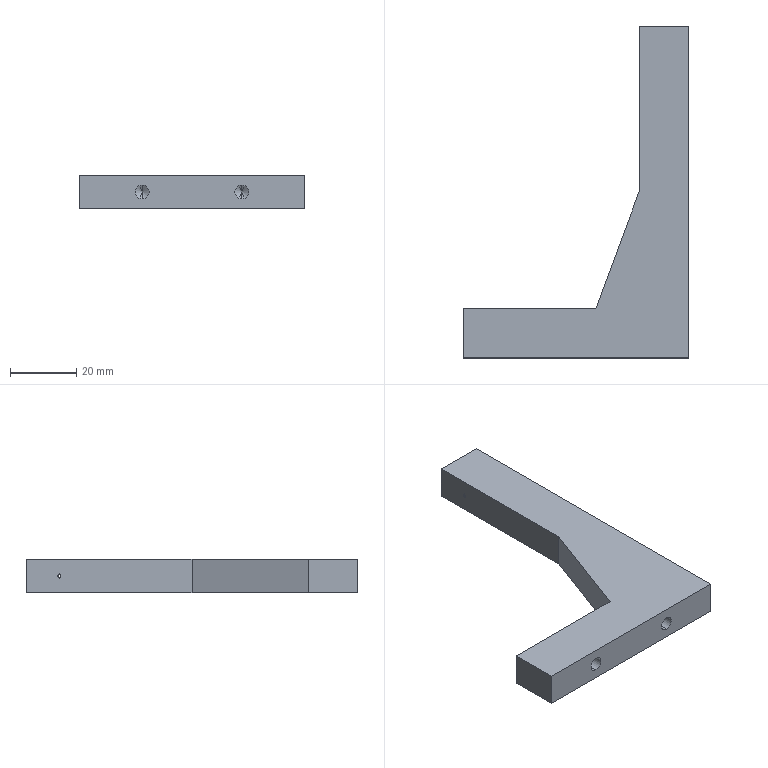Part | SolidWorks | features HoleWzd 3, Extrusion 1 | 1 solid | 33 faces | box 68 x 100 x 10 mm | volume 24328 mm3 | cylinder 12 | cone 12 | plane 9 | commonest cylinder face diameters 4.2 x8 2.5 x4
STEP:
#1=CARTESIAN_POINT('',(-58.,2.5,-1.25));
#2=VERTEX_POINT('',#1);
#3=CARTESIAN_POINT('',(-58.,2.5,1.25));
#4=VERTEX_POINT('',#3);
#5=CARTESIAN_POINT('',(-58.,2.5,0.));
#6=DIRECTION('',(0.,1.,0.));
#7=DIRECTION('',(0.,0.,1.));
#8=AXIS2_PLACEMENT_3D('',#5,#6,#7);
#9=CIRCLE('',#8,1.25);
#10=EDGE_CURVE('',#2,#4,#9,.T.);
#11=ORIENTED_EDGE('',*,*,#10,.F.);
#12=CARTESIAN_POINT('',(-58.,15.,-1.25));
#13=VERTEX_POINT('',#12);
#14=CARTESIAN_POINT('',(-58.,15.,-1.25));
#15=DIRECTION('',(0.,1.,0.));
#16=VECTOR('',#15,1000.);
#17=LINE('',#14,#16);
#18=EDGE_CURVE('',#2,#13,#17,.T.);
#19=ORIENTED_EDGE('',*,*,#18,.T.);
#20=CARTESIAN_POINT('',(-58.,15.,1.25));
#21=VERTEX_POINT('',#20);
#22=CARTESIAN_POINT('',(-58.,15.,0.));
#23=DIRECTION('',(0.,1.,0.));
#24=DIRECTION('',(0.,0.,1.));
#25=AXIS2_PLACEMENT_3D('',#22,#23,#24);
#26=CIRCLE('',#25,1.25);
#27=EDGE_CURVE('',#13,#21,#26,.T.);
#28=ORIENTED_EDGE('',*,*,#27,.T.);
#29=CARTESIAN_POINT('',(-58.,15.,1.25));
#30=DIRECTION('',(0.,1.,0.));
#31=VECTOR('',#30,1000.);
#32=LINE('',#29,#31);
#33=EDGE_CURVE('',#4,#21,#32,.T.);
#34=ORIENTED_EDGE('',*,*,#33,.F.);
#35=EDGE_LOOP('',(#11,#19,#28,#34));
#36=FACE_OUTER_BOUND('',#35,.T.);
#37=CARTESIAN_POINT('',(-58.,15.,0.));
#38=DIRECTION('',(0.,1.,0.));
#39=DIRECTION('',(0.,0.,1.));
#40=AXIS2_PLACEMENT_3D('',#37,#38,#39);
#41=CYLINDRICAL_SURFACE('',#40,1.25);
#42=ADVANCED_FACE('',(#36),#41,.F.);
#43=CARTESIAN_POINT('',(-58.,1.749,0.));
#44=VERTEX_POINT('',#43);
#45=CARTESIAN_POINT('',(-58.,2.5,1.25));
#46=DIRECTION('',(0.,0.515,0.8572));
#47=VECTOR('',#46,1000.);
#48=LINE('',#45,#47);
#49=EDGE_CURVE('',#44,#4,#48,.T.);
#50=ORIENTED_EDGE('',*,*,#49,.F.);
#51=CARTESIAN_POINT('',(-58.,2.5,-1.25));
#52=DIRECTION('',(0.,0.515,-0.8572));
#53=VECTOR('',#52,1000.);
#54=LINE('',#51,#53);
#55=EDGE_CURVE('',#44,#2,#54,.T.);
#56=ORIENTED_EDGE('',*,*,#55,.T.);
#57=ORIENTED_EDGE('',*,*,#10,.T.);
#58=EDGE_LOOP('',(#50,#56,#57));
#59=FACE_OUTER_BOUND('',#58,.T.);
#60=CARTESIAN_POINT('',(-58.,2.5,0.));
#61=DIRECTION('',(0.,1.,0.));
#62=DIRECTION('',(0.,0.,1.));
#63=AXIS2_PLACEMENT_3D('',#60,#61,#62);
#64=CONICAL_SURFACE('',#63,1.25,1.03);
#65=ADVANCED_FACE('',(#59),#64,.F.);
#66=CARTESIAN_POINT('',(-38.,2.5,-1.25));
#67=VERTEX_POINT('',#66);
#68=CARTESIAN_POINT('',(-38.,2.5,1.25));
#69=VERTEX_POINT('',#68);
#70=CARTESIAN_POINT('',(-38.,2.5,0.));
#71=DIRECTION('',(0.,1.,0.));
#72=DIRECTION('',(0.,0.,1.));
#73=AXIS2_PLACEMENT_3D('',#70,#71,#72);
#74=CIRCLE('',#73,1.25);
#75=EDGE_CURVE('',#67,#69,#74,.T.);
#76=ORIENTED_EDGE('',*,*,#75,.F.);
#77=CARTESIAN_POINT('',(-38.,15.,-1.25));
#78=VERTEX_POINT('',#77);
#79=CARTESIAN_POINT('',(-38.,15.,-1.25));
#80=DIRECTION('',(0.,1.,0.));
#81=VECTOR('',#80,1000.);
#82=LINE('',#79,#81);
#83=EDGE_CURVE('',#67,#78,#82,.T.);
#84=ORIENTED_EDGE('',*,*,#83,.T.);
#85=CARTESIAN_POINT('',(-38.,15.,1.25));
#86=VERTEX_POINT('',#85);
#87=CARTESIAN_POINT('',(-38.,15.,0.));
#88=DIRECTION('',(0.,1.,0.));
#89=DIRECTION('',(0.,0.,1.));
#90=AXIS2_PLACEMENT_3D('',#87,#88,#89);
#91=CIRCLE('',#90,1.25);
#92=EDGE_CURVE('',#78,#86,#91,.T.);
#93=ORIENTED_EDGE('',*,*,#92,.T.);
#94=CARTESIAN_POINT('',(-38.,15.,1.25));
#95=DIRECTION('',(0.,1.,0.));
#96=VECTOR('',#95,1000.);
#97=LINE('',#94,#96);
#98=EDGE_CURVE('',#69,#86,#97,.T.);
#99=ORIENTED_EDGE('',*,*,#98,.F.);
#100=EDGE_LOOP('',(#76,#84,#93,#99));
#101=FACE_OUTER_BOUND('',#100,.T.);
#102=CARTESIAN_POINT('',(-38.,15.,0.));
#103=DIRECTION('',(0.,1.,0.));
#104=DIRECTION('',(0.,0.,1.));
#105=AXIS2_PLACEMENT_3D('',#102,#103,#104);
#106=CYLINDRICAL_SURFACE('',#105,1.25);
#107=ADVANCED_FACE('',(#101),#106,.F.);
#108=CARTESIAN_POINT('',(-38.,1.749,0.));
#109=VERTEX_POINT('',#108);
#110=CARTESIAN_POINT('',(-38.,2.5,1.25));
#111=DIRECTION('',(0.,0.515,0.8572));
#112=VECTOR('',#111,1000.);
#113=LINE('',#110,#112);
#114=EDGE_CURVE('',#109,#69,#113,.T.);
#115=ORIENTED_EDGE('',*,*,#114,.F.);
#116=CARTESIAN_POINT('',(-38.,2.5,-1.25));
#117=DIRECTION('',(0.,0.515,-0.8572));
#118=VECTOR('',#117,1000.);
#119=LINE('',#116,#118);
#120=EDGE_CURVE('',#109,#67,#119,.T.);
#121=ORIENTED_EDGE('',*,*,#120,.T.);
#122=ORIENTED_EDGE('',*,*,#75,.T.);
#123=EDGE_LOOP('',(#115,#121,#122));
#124=FACE_OUTER_BOUND('',#123,.T.);
#125=CARTESIAN_POINT('',(-38.,2.5,0.));
#126=DIRECTION('',(0.,1.,0.));
#127=DIRECTION('',(0.,0.,1.));
#128=AXIS2_PLACEMENT_3D('',#125,#126,#127);
#129=CONICAL_SURFACE('',#128,1.25,1.03);
#130=ADVANCED_FACE('',(#124),#129,.F.);
#131=CARTESIAN_POINT('',(-14.,30.,2.1));
#132=VERTEX_POINT('',#131);
#133=CARTESIAN_POINT('',(-14.,30.,-2.1));
#134=VERTEX_POINT('',#133);
#135=CARTESIAN_POINT('',(-14.,30.,0.));
#136=DIRECTION('',(1.,0.,0.));
#137=DIRECTION('',(0.,0.,-1.));
#138=AXIS2_PLACEMENT_3D('',#135,#136,#137);
#139=CIRCLE('',#138,2.1);
#140=EDGE_CURVE('',#132,#134,#139,.T.);
#141=ORIENTED_EDGE('',*,*,#140,.F.);
#142=CARTESIAN_POINT('',(0.,30.,2.1));
#143=VERTEX_POINT('',#142);
#144=CARTESIAN_POINT('',(0.,30.,2.1));
#145=DIRECTION('',(1.,0.,0.));
#146=VECTOR('',#145,1000.);
#147=LINE('',#144,#146);
#148=EDGE_CURVE('',#132,#143,#147,.T.);
#149=ORIENTED_EDGE('',*,*,#148,.T.);
#150=CARTESIAN_POINT('',(0.,30.,-2.1));
#151=VERTEX_POINT('',#150);
#152=CARTESIAN_POINT('',(0.,30.,0.));
#153=DIRECTION('',(1.,0.,0.));
#154=DIRECTION('',(0.,0.,-1.));
#155=AXIS2_PLACEMENT_3D('',#152,#153,#154);
#156=CIRCLE('',#155,2.1);
#157=EDGE_CURVE('',#143,#151,#156,.T.);
#158=ORIENTED_EDGE('',*,*,#157,.T.);
#159=CARTESIAN_POINT('',(0.,30.,-2.1));
#160=DIRECTION('',(1.,0.,0.));
#161=VECTOR('',#160,1000.);
#162=LINE('',#159,#161);
#163=EDGE_CURVE('',#134,#151,#162,.T.);
#164=ORIENTED_EDGE('',*,*,#163,.F.);
#165=EDGE_LOOP('',(#141,#149,#158,#164));
#166=FACE_OUTER_BOUND('',#165,.T.);
#167=CARTESIAN_POINT('',(0.,30.,0.));
#168=DIRECTION('',(1.,0.,0.));
#169=DIRECTION('',(0.,0.,-1.));
#170=AXIS2_PLACEMENT_3D('',#167,#168,#169);
#171=CYLINDRICAL_SURFACE('',#170,2.1);
#172=ADVANCED_FACE('',(#166),#171,.F.);
#173=CARTESIAN_POINT('',(-15.262,30.,0.));
#174=VERTEX_POINT('',#173);
#175=CARTESIAN_POINT('',(-14.,30.,-2.1));
#176=DIRECTION('',(0.515,0.,-0.8572));
#177=VECTOR('',#176,1000.);
#178=LINE('',#175,#177);
#179=EDGE_CURVE('',#174,#134,#178,.T.);
#180=ORIENTED_EDGE('',*,*,#179,.F.);
#181=CARTESIAN_POINT('',(-14.,30.,2.1));
#182=DIRECTION('',(0.515,0.,0.8572));
#183=VECTOR('',#182,1000.);
#184=LINE('',#181,#183);
#185=EDGE_CURVE('',#174,#132,#184,.T.);
#186=ORIENTED_EDGE('',*,*,#185,.T.);
#187=ORIENTED_EDGE('',*,*,#140,.T.);
#188=EDGE_LOOP('',(#180,#186,#187));
#189=FACE_OUTER_BOUND('',#188,.T.);
#190=CARTESIAN_POINT('',(-14.,30.,0.));
#191=DIRECTION('',(1.,0.,0.));
#192=DIRECTION('',(0.,0.,-1.));
#193=AXIS2_PLACEMENT_3D('',#190,#191,#192);
#194=CONICAL_SURFACE('',#193,2.1,1.03);
#195=ADVANCED_FACE('',(#189),#194,.F.);
#196=CARTESIAN_POINT('',(-14.,90.,2.1));
#197=VERTEX_POINT('',#196);
#198=CARTESIAN_POINT('',(-14.,90.,-2.1));
#199=VERTEX_POINT('',#198);
#200=CARTESIAN_POINT('',(-14.,90.,0.));
#201=DIRECTION('',(1.,0.,0.));
#202=DIRECTION('',(0.,0.,-1.));
#203=AXIS2_PLACEMENT_3D('',#200,#201,#202);
#204=CIRCLE('',#203,2.1);
#205=EDGE_CURVE('',#197,#199,#204,.T.);
#206=ORIENTED_EDGE('',*,*,#205,.F.);
#207=CARTESIAN_POINT('',(0.,90.,2.1));
#208=VERTEX_POINT('',#207);
#209=CARTESIAN_POINT('',(0.,90.,2.1));
#210=DIRECTION('',(1.,0.,0.));
#211=VECTOR('',#210,1000.);
#212=LINE('',#209,#211);
#213=EDGE_CURVE('',#197,#208,#212,.T.);
#214=ORIENTED_EDGE('',*,*,#213,.T.);
#215=CARTESIAN_POINT('',(0.,90.,-2.1));
#216=VERTEX_POINT('',#215);
#217=CARTESIAN_POINT('',(0.,90.,0.));
#218=DIRECTION('',(1.,0.,0.));
#219=DIRECTION('',(0.,0.,-1.));
#220=AXIS2_PLACEMENT_3D('',#217,#218,#219);
#221=CIRCLE('',#220,2.1);
#222=EDGE_CURVE('',#208,#216,#221,.T.);
#223=ORIENTED_EDGE('',*,*,#222,.T.);
#224=CARTESIAN_POINT('',(0.,90.,-2.1));
#225=DIRECTION('',(1.,0.,0.));
#226=VECTOR('',#225,1000.);
#227=LINE('',#224,#226);
#228=EDGE_CURVE('',#199,#216,#227,.T.);
#229=ORIENTED_EDGE('',*,*,#228,.F.);
#230=EDGE_LOOP('',(#206,#214,#223,#229));
#231=FACE_OUTER_BOUND('',#230,.T.);
#232=CARTESIAN_POINT('',(0.,90.,0.));
#233=DIRECTION('',(1.,0.,0.));
#234=DIRECTION('',(0.,0.,-1.));
#235=AXIS2_PLACEMENT_3D('',#232,#233,#234);
#236=CYLINDRICAL_SURFACE('',#235,2.1);
#237=ADVANCED_FACE('',(#231),#236,.F.);
#238=CARTESIAN_POINT('',(-15.,90.,0.4357));
#239=VERTEX_POINT('',#238);
#240=CARTESIAN_POINT('',(-15.,90.,-0.4357));
#241=VERTEX_POINT('',#240);
#242=CARTESIAN_POINT('',(-15.,90.,0.));
#243=DIRECTION('',(1.,0.,0.));
#244=DIRECTION('',(0.,0.,-1.));
#245=AXIS2_PLACEMENT_3D('',#242,#243,#244);
#246=CIRCLE('',#245,0.4357);
#247=EDGE_CURVE('',#239,#241,#246,.T.);
#248=ORIENTED_EDGE('',*,*,#247,.F.);
#249=CARTESIAN_POINT('',(-14.,90.,2.1));
#250=DIRECTION('',(0.515,0.,0.8572));
#251=VECTOR('',#250,1000.);
#252=LINE('',#249,#251);
#253=EDGE_CURVE('',#239,#197,#252,.T.);
#254=ORIENTED_EDGE('',*,*,#253,.T.);
#255=ORIENTED_EDGE('',*,*,#205,.T.);
#256=CARTESIAN_POINT('',(-14.,90.,-2.1));
#257=DIRECTION('',(0.515,0.,-0.8572));
#258=VECTOR('',#257,1000.);
#259=LINE('',#256,#258);
#260=EDGE_CURVE('',#241,#199,#259,.T.);
#261=ORIENTED_EDGE('',*,*,#260,.F.);
#262=EDGE_LOOP('',(#248,#254,#255,#261));
#263=FACE_OUTER_BOUND('',#262,.T.);
#264=CARTESIAN_POINT('',(-14.,90.,0.));
#265=DIRECTION('',(1.,0.,0.));
#266=DIRECTION('',(0.,0.,-1.));
#267=AXIS2_PLACEMENT_3D('',#264,#265,#266);
#268=CONICAL_SURFACE('',#267,2.1,1.03);
#269=ADVANCED_FACE('',(#263),#268,.F.);
#270=CARTESIAN_POINT('',(-49.,13.,2.1));
#271=VERTEX_POINT('',#270);
#272=CARTESIAN_POINT('',(-49.,13.,-2.1));
#273=VERTEX_POINT('',#272);
#274=CARTESIAN_POINT('',(-49.,13.,0.));
#275=DIRECTION('',(0.,-1.,0.));
#276=DIRECTION('',(0.,0.,-1.));
#277=AXIS2_PLACEMENT_3D('',#274,#275,#276);
#278=CIRCLE('',#277,2.1);
#279=EDGE_CURVE('',#271,#273,#278,.T.);
#280=ORIENTED_EDGE('',*,*,#279,.F.);
#281=CARTESIAN_POINT('',(-49.,0.,2.1));
#282=VERTEX_POINT('',#281);
#283=CARTESIAN_POINT('',(-49.,0.,2.1));
#284=DIRECTION('',(0.,-1.,0.));
#285=VECTOR('',#284,1000.);
#286=LINE('',#283,#285);
#287=EDGE_CURVE('',#271,#282,#286,.T.);
#288=ORIENTED_EDGE('',*,*,#287,.T.);
#289=CARTESIAN_POINT('',(-49.,0.,-2.1));
#290=VERTEX_POINT('',#289);
#291=CARTESIAN_POINT('',(-49.,0.,0.));
#292=DIRECTION('',(0.,-1.,0.));
#293=DIRECTION('',(0.,0.,-1.));
#294=AXIS2_PLACEMENT_3D('',#291,#292,#293);
#295=CIRCLE('',#294,2.1);
#296=EDGE_CURVE('',#282,#290,#295,.T.);
#297=ORIENTED_EDGE('',*,*,#296,.T.);
#298=CARTESIAN_POINT('',(-49.,0.,-2.1));
#299=DIRECTION('',(0.,-1.,0.));
#300=VECTOR('',#299,1000.);
#301=LINE('',#298,#300);
#302=EDGE_CURVE('',#273,#290,#301,.T.);
#303=ORIENTED_EDGE('',*,*,#302,.F.);
#304=EDGE_LOOP('',(#280,#288,#297,#303));
#305=FACE_OUTER_BOUND('',#304,.T.);
#306=CARTESIAN_POINT('',(-49.,0.,0.));
#307=DIRECTION('',(0.,-1.,0.));
#308=DIRECTION('',(0.,0.,-1.));
#309=AXIS2_PLACEMENT_3D('',#306,#307,#308);
#310=CYLINDRICAL_SURFACE('',#309,2.1);
#311=ADVANCED_FACE('',(#305),#310,.F.);
#312=CARTESIAN_POINT('',(-49.,14.262,0.));
#313=VERTEX_POINT('',#312);
#314=CARTESIAN_POINT('',(-49.,13.,-2.1));
#315=DIRECTION('',(0.,-0.515,-0.8572));
#316=VECTOR('',#315,1000.);
#317=LINE('',#314,#316);
#318=EDGE_CURVE('',#313,#273,#317,.T.);
#319=ORIENTED_EDGE('',*,*,#318,.F.);
#320=CARTESIAN_POINT('',(-49.,13.,2.1));
#321=DIRECTION('',(0.,-0.515,0.8572));
#322=VECTOR('',#321,1000.);
#323=LINE('',#320,#322);
#324=EDGE_CURVE('',#313,#271,#323,.T.);
#325=ORIENTED_EDGE('',*,*,#324,.T.);
#326=ORIENTED_EDGE('',*,*,#279,.T.);
#327=EDGE_LOOP('',(#319,#325,#326));
#328=FACE_OUTER_BOUND('',#327,.T.);
#329=CARTESIAN_POINT('',(-49.,13.,0.));
#330=DIRECTION('',(0.,-1.,0.));
#331=DIRECTION('',(0.,0.,-1.));
#332=AXIS2_PLACEMENT_3D('',#329,#330,#331);
#333=CONICAL_SURFACE('',#332,2.1,1.03);
#334=ADVANCED_FACE('',(#328),#333,.F.);
#335=CARTESIAN_POINT('',(-19.,13.,2.1));
#336=VERTEX_POINT('',#335);
#337=CARTESIAN_POINT('',(-19.,13.,-2.1));
#338=VERTEX_POINT('',#337);
#339=CARTESIAN_POINT('',(-19.,13.,0.));
#340=DIRECTION('',(0.,-1.,0.));
#341=DIRECTION('',(0.,0.,-1.));
#342=AXIS2_PLACEMENT_3D('',#339,#340,#341);
#343=CIRCLE('',#342,2.1);
#344=EDGE_CURVE('',#336,#338,#343,.T.);
#345=ORIENTED_EDGE('',*,*,#344,.F.);
#346=CARTESIAN_POINT('',(-19.,0.,2.1));
#347=VERTEX_POINT('',#346);
#348=CARTESIAN_POINT('',(-19.,0.,2.1));
#349=DIRECTION('',(0.,-1.,0.));
#350=VECTOR('',#349,1000.);
#351=LINE('',#348,#350);
#352=EDGE_CURVE('',#336,#347,#351,.T.);
#353=ORIENTED_EDGE('',*,*,#352,.T.);
#354=CARTESIAN_POINT('',(-19.,0.,-2.1));
#355=VERTEX_POINT('',#354);
#356=CARTESIAN_POINT('',(-19.,0.,0.));
#357=DIRECTION('',(0.,-1.,0.));
#358=DIRECTION('',(0.,0.,-1.));
#359=AXIS2_PLACEMENT_3D('',#356,#357,#358);
#360=CIRCLE('',#359,2.1);
#361=EDGE_CURVE('',#347,#355,#360,.T.);
#362=ORIENTED_EDGE('',*,*,#361,.T.);
#363=CARTESIAN_POINT('',(-19.,0.,-2.1));
#364=DIRECTION('',(0.,-1.,0.));
#365=VECTOR('',#364,1000.);
#366=LINE('',#363,#365);
#367=EDGE_CURVE('',#338,#355,#366,.T.);
#368=ORIENTED_EDGE('',*,*,#367,.F.);
#369=EDGE_LOOP('',(#345,#353,#362,#368));
#370=FACE_OUTER_BOUND('',#369,.T.);
#371=CARTESIAN_POINT('',(-19.,0.,0.));
#372=DIRECTION('',(0.,-1.,0.));
#373=DIRECTION('',(0.,0.,-1.));
#374=AXIS2_PLACEMENT_3D('',#371,#372,#373);
#375=CYLINDRICAL_SURFACE('',#374,2.1);
#376=ADVANCED_FACE('',(#370),#375,.F.);
#377=CARTESIAN_POINT('',(-19.,14.262,0.));
#378=VERTEX_POINT('',#377);
#379=CARTESIAN_POINT('',(-19.,13.,-2.1));
#380=DIRECTION('',(0.,-0.515,-0.8572));
#381=VECTOR('',#380,1000.);
#382=LINE('',#379,#381);
#383=EDGE_CURVE('',#378,#338,#382,.T.);
#384=ORIENTED_EDGE('',*,*,#383,.F.);
#385=CARTESIAN_POINT('',(-19.,13.,2.1));
#386=DIRECTION('',(0.,-0.515,0.8572));
#387=VECTOR('',#386,1000.);
#388=LINE('',#385,#387);
#389=EDGE_CURVE('',#378,#336,#388,.T.);
#390=ORIENTED_EDGE('',*,*,#389,.T.);
#391=ORIENTED_EDGE('',*,*,#344,.T.);
#392=EDGE_LOOP('',(#384,#390,#391));
#393=FACE_OUTER_BOUND('',#392,.T.);
#394=CARTESIAN_POINT('',(-19.,13.,0.));
#395=DIRECTION('',(0.,-1.,0.));
#396=DIRECTION('',(0.,0.,-1.));
#397=AXIS2_PLACEMENT_3D('',#394,#395,#396);
#398=CONICAL_SURFACE('',#397,2.1,1.03);
#399=ADVANCED_FACE('',(#393),#398,.F.);
#400=CARTESIAN_POINT('',(-49.,0.,0.));
#401=DIRECTION('',(0.,-1.,0.));
#402=DIRECTION('',(0.,0.,-1.));
#403=AXIS2_PLACEMENT_3D('',#400,#401,#402);
#404=CIRCLE('',#403,2.1);
#405=EDGE_CURVE('',#290,#282,#404,.T.);
#406=ORIENTED_EDGE('',*,*,#405,.F.);
#407=ORIENTED_EDGE('',*,*,#296,.F.);
#408=EDGE_LOOP('',(#406,#407));
#409=FACE_BOUND('',#408,.T.);
#410=CARTESIAN_POINT('',(-19.,0.,0.));
#411=DIRECTION('',(0.,-1.,0.));
#412=DIRECTION('',(0.,0.,-1.));
#413=AXIS2_PLACEMENT_3D('',#410,#411,#412);
#414=CIRCLE('',#413,2.1);
#415=EDGE_CURVE('',#355,#347,#414,.T.);
#416=ORIENTED_EDGE('',*,*,#415,.F.);
#417=ORIENTED_EDGE('',*,*,#361,.F.);
#418=EDGE_LOOP('',(#416,#417));
#419=FACE_BOUND('',#418,.T.);
#420=CARTESIAN_POINT('',(-68.,0.,-5.));
#421=VERTEX_POINT('',#420);
#422=CARTESIAN_POINT('',(0.,0.,-5.));
#423=VERTEX_POINT('',#422);
#424=CARTESIAN_POINT('',(0.,0.,-5.));
#425=DIRECTION('',(1.,0.,0.));
#426=VECTOR('',#425,1000.);
#427=LINE('',#424,#426);
#428=EDGE_CURVE('',#421,#423,#427,.T.);
#429=ORIENTED_EDGE('',*,*,#428,.T.);
#430=CARTESIAN_POINT('',(0.,0.,5.));
#431=VERTEX_POINT('',#430);
#432=CARTESIAN_POINT('',(0.,0.,5.));
#433=DIRECTION('',(0.,0.,-1.));
#434=VECTOR('',#433,1000.);
#435=LINE('',#432,#434);
#436=EDGE_CURVE('',#431,#423,#435,.T.);
#437=ORIENTED_EDGE('',*,*,#436,.F.);
#438=CARTESIAN_POINT('',(-68.,0.,5.));
#439=VERTEX_POINT('',#438);
#440=CARTESIAN_POINT('',(0.,0.,5.));
#441=DIRECTION('',(1.,0.,0.));
#442=VECTOR('',#441,1000.);
#443=LINE('',#440,#442);
#444=EDGE_CURVE('',#439,#431,#443,.T.);
#445=ORIENTED_EDGE('',*,*,#444,.F.);
#446=CARTESIAN_POINT('',(-68.,0.,5.));
#447=DIRECTION('',(0.,0.,-1.));
#448=VECTOR('',#447,1000.);
#449=LINE('',#446,#448);
#450=EDGE_CURVE('',#439,#421,#449,.T.);
#451=ORIENTED_EDGE('',*,*,#450,.T.);
#452=EDGE_LOOP('',(#429,#437,#445,#451));
#453=FACE_OUTER_BOUND('',#452,.T.);
#454=CARTESIAN_POINT('',(0.,0.,5.));
#455=DIRECTION('',(0.,1.,0.));
#456=DIRECTION('',(0.,0.,1.));
#457=AXIS2_PLACEMENT_3D('',#454,#455,#456);
#458=PLANE('',#457);
#459=ADVANCED_FACE('',(#409,#419,#453),#458,.F.);
#460=CARTESIAN_POINT('',(0.,30.,0.));
#461=DIRECTION('',(1.,0.,0.));
#462=DIRECTION('',(0.,0.,-1.));
#463=AXIS2_PLACEMENT_3D('',#460,#461,#462);
#464=CIRCLE('',#463,2.1);
#465=EDGE_CURVE('',#151,#143,#464,.T.);
#466=ORIENTED_EDGE('',*,*,#465,.F.);
#467=ORIENTED_EDGE('',*,*,#157,.F.);
#468=EDGE_LOOP('',(#466,#467));
#469=FACE_BOUND('',#468,.T.);
#470=CARTESIAN_POINT('',(0.,90.,0.));
#471=DIRECTION('',(1.,0.,0.));
#472=DIRECTION('',(0.,0.,-1.));
#473=AXIS2_PLACEMENT_3D('',#470,#471,#472);
#474=CIRCLE('',#473,2.1);
#475=EDGE_CURVE('',#216,#208,#474,.T.);
#476=ORIENTED_EDGE('',*,*,#475,.F.);
#477=ORIENTED_EDGE('',*,*,#222,.F.);
#478=EDGE_LOOP('',(#476,#477));
#479=FACE_BOUND('',#478,.T.);
#480=CARTESIAN_POINT('',(0.,100.,-5.));
#481=VERTEX_POINT('',#480);
#482=CARTESIAN_POINT('',(0.,100.,-5.));
#483=DIRECTION('',(0.,1.,0.));
#484=VECTOR('',#483,1000.);
#485=LINE('',#482,#484);
#486=EDGE_CURVE('',#423,#481,#485,.T.);
#487=ORIENTED_EDGE('',*,*,#486,.T.);
#488=CARTESIAN_POINT('',(0.,100.,5.));
#489=VERTEX_POINT('',#488);
#490=CARTESIAN_POINT('',(0.,100.,5.));
#491=DIRECTION('',(0.,0.,-1.));
#492=VECTOR('',#491,1000.);
#493=LINE('',#490,#492);
#494=EDGE_CURVE('',#489,#481,#493,.T.);
#495=ORIENTED_EDGE('',*,*,#494,.F.);
#496=CARTESIAN_POINT('',(0.,100.,5.));
#497=DIRECTION('',(0.,1.,0.));
#498=VECTOR('',#497,1000.);
#499=LINE('',#496,#498);
#500=EDGE_CURVE('',#431,#489,#499,.T.);
#501=ORIENTED_EDGE('',*,*,#500,.F.);
#502=ORIENTED_EDGE('',*,*,#436,.T.);
#503=EDGE_LOOP('',(#487,#495,#501,#502));
#504=FACE_OUTER_BOUND('',#503,.T.);
#505=CARTESIAN_POINT('',(0.,100.,5.));
#506=DIRECTION('',(-1.,0.,0.));
#507=DIRECTION('',(0.,-1.,0.));
#508=AXIS2_PLACEMENT_3D('',#505,#506,#507);
#509=PLANE('',#508);
#510=ADVANCED_FACE('',(#469,#479,#504),#509,.F.);
#511=CARTESIAN_POINT('',(-15.,100.,-5.));
#512=VERTEX_POINT('',#511);
#513=CARTESIAN_POINT('',(-15.,100.,-5.));
#514=DIRECTION('',(-1.,0.,0.));
#515=VECTOR('',#514,1000.);
#516=LINE('',#513,#515);
#517=EDGE_CURVE('',#481,#512,#516,.T.);
#518=ORIENTED_EDGE('',*,*,#517,.T.);
#519=CARTESIAN_POINT('',(-15.,100.,5.));
#520=VERTEX_POINT('',#519);
#521=CARTESIAN_POINT('',(-15.,100.,5.));
#522=DIRECTION('',(0.,0.,-1.));
#523=VECTOR('',#522,1000.);
#524=LINE('',#521,#523);
#525=EDGE_CURVE('',#520,#512,#524,.T.);
#526=ORIENTED_EDGE('',*,*,#525,.F.);
#527=CARTESIAN_POINT('',(-15.,100.,5.));
#528=DIRECTION('',(-1.,0.,0.));
#529=VECTOR('',#528,1000.);
#530=LINE('',#527,#529);
#531=EDGE_CURVE('',#489,#520,#530,.T.);
#532=ORIENTED_EDGE('',*,*,#531,.F.);
#533=ORIENTED_EDGE('',*,*,#494,.T.);
#534=EDGE_LOOP('',(#518,#526,#532,#533));
#535=FACE_OUTER_BOUND('',#534,.T.);
#536=CARTESIAN_POINT('',(-15.,100.,5.));
#537=DIRECTION('',(0.,-1.,0.));
#538=DIRECTION('',(0.,0.,-1.));
#539=AXIS2_PLACEMENT_3D('',#536,#537,#538);
#540=PLANE('',#539);
#541=ADVANCED_FACE('',(#535),#540,.F.);
#542=CARTESIAN_POINT('',(-15.,90.,0.));
#543=DIRECTION('',(1.,0.,0.));
#544=DIRECTION('',(0.,0.,-1.));
#545=AXIS2_PLACEMENT_3D('',#542,#543,#544);
#546=CIRCLE('',#545,0.4357);
#547=EDGE_CURVE('',#241,#239,#546,.T.);
#548=ORIENTED_EDGE('',*,*,#547,.T.);
#549=ORIENTED_EDGE('',*,*,#247,.T.);
#550=EDGE_LOOP('',(#548,#549));
#551=FACE_BOUND('',#550,.T.);
#552=CARTESIAN_POINT('',(-15.,50.,-5.));
#553=VERTEX_POINT('',#552);
#554=CARTESIAN_POINT('',(-15.,50.,-5.));
#555=DIRECTION('',(0.,-1.,0.));
#556=VECTOR('',#555,1000.);
#557=LINE('',#554,#556);
#558=EDGE_CURVE('',#512,#553,#557,.T.);
#559=ORIENTED_EDGE('',*,*,#558,.T.);
#560=CARTESIAN_POINT('',(-15.,50.,5.));
#561=VERTEX_POINT('',#560);
#562=CARTESIAN_POINT('',(-15.,50.,5.));
#563=DIRECTION('',(0.,0.,-1.));
#564=VECTOR('',#563,1000.);
#565=LINE('',#562,#564);
#566=EDGE_CURVE('',#561,#553,#565,.T.);
#567=ORIENTED_EDGE('',*,*,#566,.F.);
#568=CARTESIAN_POINT('',(-15.,50.,5.));
#569=DIRECTION('',(0.,-1.,0.));
#570=VECTOR('',#569,1000.);
#571=LINE('',#568,#570);
#572=EDGE_CURVE('',#520,#561,#571,.T.);
#573=ORIENTED_EDGE('',*,*,#572,.F.);
#574=ORIENTED_EDGE('',*,*,#525,.T.);
#575=EDGE_LOOP('',(#559,#567,#573,#574));
#576=FACE_OUTER_BOUND('',#575,.T.);
#577=CARTESIAN_POINT('',(-15.,50.,5.));
#578=DIRECTION('',(1.,0.,0.));
#579=DIRECTION('',(0.,0.,-1.));
#580=AXIS2_PLACEMENT_3D('',#577,#578,#579);
#581=PLANE('',#580);
#582=ADVANCED_FACE('',(#551,#576),#581,.F.);
#583=CARTESIAN_POINT('',(-28.,15.,-5.));
#584=VERTEX_POINT('',#583);
#585=CARTESIAN_POINT('',(-28.,15.,-5.));
#586=DIRECTION('',(-0.3482,-0.9374,0.));
#587=VECTOR('',#586,1000.);
#588=LINE('',#585,#587);
#589=EDGE_CURVE('',#553,#584,#588,.T.);
#590=ORIENTED_EDGE('',*,*,#589,.T.);
#591=CARTESIAN_POINT('',(-28.,15.,5.));
#592=VERTEX_POINT('',#591);
#593=CARTESIAN_POINT('',(-28.,15.,5.));
#594=DIRECTION('',(0.,0.,-1.));
#595=VECTOR('',#594,1000.);
#596=LINE('',#593,#595);
#597=EDGE_CURVE('',#592,#584,#596,.T.);
#598=ORIENTED_EDGE('',*,*,#597,.F.);
#599=CARTESIAN_POINT('',(-28.,15.,5.));
#600=DIRECTION('',(-0.3482,-0.9374,0.));
#601=VECTOR('',#600,1000.);
#602=LINE('',#599,#601);
#603=EDGE_CURVE('',#561,#592,#602,.T.);
#604=ORIENTED_EDGE('',*,*,#603,.F.);
#605=ORIENTED_EDGE('',*,*,#566,.T.);
#606=EDGE_LOOP('',(#590,#598,#604,#605));
#607=FACE_OUTER_BOUND('',#606,.T.);
#608=CARTESIAN_POINT('',(-28.,15.,5.));
#609=DIRECTION('',(0.9374,-0.3482,0.));
#610=DIRECTION('',(0.3482,0.9374,0.));
#611=AXIS2_PLACEMENT_3D('',#608,#609,#610);
#612=PLANE('',#611);
#613=ADVANCED_FACE('',(#607),#612,.F.);
#614=CARTESIAN_POINT('',(-58.,15.,0.));
#615=DIRECTION('',(0.,1.,0.));
#616=DIRECTION('',(0.,0.,1.));
#617=AXIS2_PLACEMENT_3D('',#614,#615,#616);
#618=CIRCLE('',#617,1.25);
#619=EDGE_CURVE('',#21,#13,#618,.T.);
#620=ORIENTED_EDGE('',*,*,#619,.F.);
#621=ORIENTED_EDGE('',*,*,#27,.F.);
#622=EDGE_LOOP('',(#620,#621));
#623=FACE_BOUND('',#622,.T.);
#624=CARTESIAN_POINT('',(-38.,15.,0.));
#625=DIRECTION('',(0.,1.,0.));
#626=DIRECTION('',(0.,0.,1.));
#627=AXIS2_PLACEMENT_3D('',#624,#625,#626);
#628=CIRCLE('',#627,1.25);
#629=EDGE_CURVE('',#86,#78,#628,.T.);
#630=ORIENTED_EDGE('',*,*,#629,.F.);
#631=ORIENTED_EDGE('',*,*,#92,.F.);
#632=EDGE_LOOP('',(#630,#631));
#633=FACE_BOUND('',#632,.T.);
#634=CARTESIAN_POINT('',(-68.,15.,-5.));
#635=VERTEX_POINT('',#634);
#636=CARTESIAN_POINT('',(-68.,15.,-5.));
#637=DIRECTION('',(-1.,0.,0.));
#638=VECTOR('',#637,1000.);
#639=LINE('',#636,#638);
#640=EDGE_CURVE('',#584,#635,#639,.T.);
#641=ORIENTED_EDGE('',*,*,#640,.T.);
#642=CARTESIAN_POINT('',(-68.,15.,5.));
#643=VERTEX_POINT('',#642);
#644=CARTESIAN_POINT('',(-68.,15.,5.));
#645=DIRECTION('',(0.,0.,-1.));
#646=VECTOR('',#645,1000.);
#647=LINE('',#644,#646);
#648=EDGE_CURVE('',#643,#635,#647,.T.);
#649=ORIENTED_EDGE('',*,*,#648,.F.);
#650=CARTESIAN_POINT('',(-68.,15.,5.));
#651=DIRECTION('',(-1.,0.,0.));
#652=VECTOR('',#651,1000.);
#653=LINE('',#650,#652);
#654=EDGE_CURVE('',#592,#643,#653,.T.);
#655=ORIENTED_EDGE('',*,*,#654,.F.);
#656=ORIENTED_EDGE('',*,*,#597,.T.);
#657=EDGE_LOOP('',(#641,#649,#655,#656));
#658=FACE_OUTER_BOUND('',#657,.T.);
#659=CARTESIAN_POINT('',(-68.,15.,5.));
#660=DIRECTION('',(0.,-1.,0.));
#661=DIRECTION('',(0.,0.,-1.));
#662=AXIS2_PLACEMENT_3D('',#659,#660,#661);
#663=PLANE('',#662);
#664=ADVANCED_FACE('',(#623,#633,#658),#663,.F.);
#665=CARTESIAN_POINT('',(-68.,0.,-5.));
#666=DIRECTION('',(0.,-1.,0.));
#667=VECTOR('',#666,1000.);
#668=LINE('',#665,#667);
#669=EDGE_CURVE('',#635,#421,#668,.T.);
#670=ORIENTED_EDGE('',*,*,#669,.T.);
#671=ORIENTED_EDGE('',*,*,#450,.F.);
#672=CARTESIAN_POINT('',(-68.,0.,5.));
#673=DIRECTION('',(0.,-1.,0.));
#674=VECTOR('',#673,1000.);
#675=LINE('',#672,#674);
#676=EDGE_CURVE('',#643,#439,#675,.T.);
#677=ORIENTED_EDGE('',*,*,#676,.F.);
#678=ORIENTED_EDGE('',*,*,#648,.T.);
#679=EDGE_LOOP('',(#670,#671,#677,#678));
#680=FACE_OUTER_BOUND('',#679,.T.);
#681=CARTESIAN_POINT('',(-68.,0.,5.));
#682=DIRECTION('',(1.,0.,0.));
#683=DIRECTION('',(0.,0.,-1.));
#684=AXIS2_PLACEMENT_3D('',#681,#682,#683);
#685=PLANE('',#684);
#686=ADVANCED_FACE('',(#680),#685,.F.);
#687=ORIENTED_EDGE('',*,*,#444,.T.);
#688=ORIENTED_EDGE('',*,*,#500,.T.);
#689=ORIENTED_EDGE('',*,*,#531,.T.);
#690=ORIENTED_EDGE('',*,*,#572,.T.);
#691=ORIENTED_EDGE('',*,*,#603,.T.);
#692=ORIENTED_EDGE('',*,*,#654,.T.);
#693=ORIENTED_EDGE('',*,*,#676,.T.);
#694=EDGE_LOOP('',(#687,#688,#689,#690,#691,#692,#693));
#695=FACE_OUTER_BOUND('',#694,.T.);
#696=CARTESIAN_POINT('',(0.,0.,5.));
#697=DIRECTION('',(0.,0.,-1.));
#698=DIRECTION('',(-1.,0.,0.));
#699=AXIS2_PLACEMENT_3D('',#696,#697,#698);
#700=PLANE('',#699);
#701=ADVANCED_FACE('',(#695),#700,.F.);
#702=ORIENTED_EDGE('',*,*,#428,.F.);
#703=ORIENTED_EDGE('',*,*,#669,.F.);
#704=ORIENTED_EDGE('',*,*,#640,.F.);
#705=ORIENTED_EDGE('',*,*,#589,.F.);
#706=ORIENTED_EDGE('',*,*,#558,.F.);
#707=ORIENTED_EDGE('',*,*,#517,.F.);
#708=ORIENTED_EDGE('',*,*,#486,.F.);
#709=EDGE_LOOP('',(#702,#703,#704,#705,#706,#707,#708));
#710=FACE_OUTER_BOUND('',#709,.T.);
#711=CARTESIAN_POINT('',(0.,0.,-5.));
#712=DIRECTION('',(0.,0.,-1.));
#713=DIRECTION('',(-1.,0.,0.));
#714=AXIS2_PLACEMENT_3D('',#711,#712,#713);
#715=PLANE('',#714);
#716=ADVANCED_FACE('',(#710),#715,.T.);
#717=ORIENTED_EDGE('',*,*,#389,.F.);
#718=ORIENTED_EDGE('',*,*,#383,.T.);
#719=CARTESIAN_POINT('',(-19.,13.,0.));
#720=DIRECTION('',(0.,-1.,0.));
#721=DIRECTION('',(0.,0.,-1.));
#722=AXIS2_PLACEMENT_3D('',#719,#720,#721);
#723=CIRCLE('',#722,2.1);
#724=EDGE_CURVE('',#338,#336,#723,.T.);
#725=ORIENTED_EDGE('',*,*,#724,.T.);
#726=EDGE_LOOP('',(#717,#718,#725));
#727=FACE_OUTER_BOUND('',#726,.T.);
#728=CARTESIAN_POINT('',(-19.,13.,0.));
#729=DIRECTION('',(0.,-1.,0.));
#730=DIRECTION('',(0.,0.,-1.));
#731=AXIS2_PLACEMENT_3D('',#728,#729,#730);
#732=CONICAL_SURFACE('',#731,2.1,1.03);
#733=ADVANCED_FACE('',(#727),#732,.F.);
#734=ORIENTED_EDGE('',*,*,#352,.F.);
#735=ORIENTED_EDGE('',*,*,#724,.F.);
#736=ORIENTED_EDGE('',*,*,#367,.T.);
#737=ORIENTED_EDGE('',*,*,#415,.T.);
#738=EDGE_LOOP('',(#734,#735,#736,#737));
#739=FACE_OUTER_BOUND('',#738,.T.);
#740=CARTESIAN_POINT('',(-19.,0.,0.));
#741=DIRECTION('',(0.,-1.,0.));
#742=DIRECTION('',(0.,0.,-1.));
#743=AXIS2_PLACEMENT_3D('',#740,#741,#742);
#744=CYLINDRICAL_SURFACE('',#743,2.1);
#745=ADVANCED_FACE('',(#739),#744,.F.);
#746=ORIENTED_EDGE('',*,*,#324,.F.);
#747=ORIENTED_EDGE('',*,*,#318,.T.);
#748=CARTESIAN_POINT('',(-49.,13.,0.));
#749=DIRECTION('',(0.,-1.,0.));
#750=DIRECTION('',(0.,0.,-1.));
#751=AXIS2_PLACEMENT_3D('',#748,#749,#750);
#752=CIRCLE('',#751,2.1);
#753=EDGE_CURVE('',#273,#271,#752,.T.);
#754=ORIENTED_EDGE('',*,*,#753,.T.);
#755=EDGE_LOOP('',(#746,#747,#754));
#756=FACE_OUTER_BOUND('',#755,.T.);
#757=CARTESIAN_POINT('',(-49.,13.,0.));
#758=DIRECTION('',(0.,-1.,0.));
#759=DIRECTION('',(0.,0.,-1.));
#760=AXIS2_PLACEMENT_3D('',#757,#758,#759);
#761=CONICAL_SURFACE('',#760,2.1,1.03);
#762=ADVANCED_FACE('',(#756),#761,.F.);
#763=ORIENTED_EDGE('',*,*,#287,.F.);
#764=ORIENTED_EDGE('',*,*,#753,.F.);
#765=ORIENTED_EDGE('',*,*,#302,.T.);
#766=ORIENTED_EDGE('',*,*,#405,.T.);
#767=EDGE_LOOP('',(#763,#764,#765,#766));
#768=FACE_OUTER_BOUND('',#767,.T.);
#769=CARTESIAN_POINT('',(-49.,0.,0.));
#770=DIRECTION('',(0.,-1.,0.));
#771=DIRECTION('',(0.,0.,-1.));
#772=AXIS2_PLACEMENT_3D('',#769,#770,#771);
#773=CYLINDRICAL_SURFACE('',#772,2.1);
#774=ADVANCED_FACE('',(#768),#773,.F.);
#775=ORIENTED_EDGE('',*,*,#253,.F.);
#776=ORIENTED_EDGE('',*,*,#547,.F.);
#777=ORIENTED_EDGE('',*,*,#260,.T.);
#778=CARTESIAN_POINT('',(-14.,90.,0.));
#779=DIRECTION('',(1.,0.,0.));
#780=DIRECTION('',(0.,0.,-1.));
#781=AXIS2_PLACEMENT_3D('',#778,#779,#780);
#782=CIRCLE('',#781,2.1);
#783=EDGE_CURVE('',#199,#197,#782,.T.);
#784=ORIENTED_EDGE('',*,*,#783,.T.);
#785=EDGE_LOOP('',(#775,#776,#777,#784));
#786=FACE_OUTER_BOUND('',#785,.T.);
#787=CARTESIAN_POINT('',(-14.,90.,0.));
#788=DIRECTION('',(1.,0.,0.));
#789=DIRECTION('',(0.,0.,-1.));
#790=AXIS2_PLACEMENT_3D('',#787,#788,#789);
#791=CONICAL_SURFACE('',#790,2.1,1.03);
#792=ADVANCED_FACE('',(#786),#791,.F.);
#793=ORIENTED_EDGE('',*,*,#213,.F.);
#794=ORIENTED_EDGE('',*,*,#783,.F.);
#795=ORIENTED_EDGE('',*,*,#228,.T.);
#796=ORIENTED_EDGE('',*,*,#475,.T.);
#797=EDGE_LOOP('',(#793,#794,#795,#796));
#798=FACE_OUTER_BOUND('',#797,.T.);
#799=CARTESIAN_POINT('',(0.,90.,0.));
#800=DIRECTION('',(1.,0.,0.));
#801=DIRECTION('',(0.,0.,-1.));
#802=AXIS2_PLACEMENT_3D('',#799,#800,#801);
#803=CYLINDRICAL_SURFACE('',#802,2.1);
#804=ADVANCED_FACE('',(#798),#803,.F.);
#805=ORIENTED_EDGE('',*,*,#185,.F.);
#806=ORIENTED_EDGE('',*,*,#179,.T.);
#807=CARTESIAN_POINT('',(-14.,30.,0.));
#808=DIRECTION('',(1.,0.,0.));
#809=DIRECTION('',(0.,0.,-1.));
#810=AXIS2_PLACEMENT_3D('',#807,#808,#809);
#811=CIRCLE('',#810,2.1);
#812=EDGE_CURVE('',#134,#132,#811,.T.);
#813=ORIENTED_EDGE('',*,*,#812,.T.);
#814=EDGE_LOOP('',(#805,#806,#813));
#815=FACE_OUTER_BOUND('',#814,.T.);
#816=CARTESIAN_POINT('',(-14.,30.,0.));
#817=DIRECTION('',(1.,0.,0.));
#818=DIRECTION('',(0.,0.,-1.));
#819=AXIS2_PLACEMENT_3D('',#816,#817,#818);
#820=CONICAL_SURFACE('',#819,2.1,1.03);
#821=ADVANCED_FACE('',(#815),#820,.F.);
#822=ORIENTED_EDGE('',*,*,#148,.F.);
#823=ORIENTED_EDGE('',*,*,#812,.F.);
#824=ORIENTED_EDGE('',*,*,#163,.T.);
#825=ORIENTED_EDGE('',*,*,#465,.T.);
#826=EDGE_LOOP('',(#822,#823,#824,#825));
#827=FACE_OUTER_BOUND('',#826,.T.);
#828=CARTESIAN_POINT('',(0.,30.,0.));
#829=DIRECTION('',(1.,0.,0.));
#830=DIRECTION('',(0.,0.,-1.));
#831=AXIS2_PLACEMENT_3D('',#828,#829,#830);
#832=CYLINDRICAL_SURFACE('',#831,2.1);
#833=ADVANCED_FACE('',(#827),#832,.F.);
#834=ORIENTED_EDGE('',*,*,#120,.F.);
#835=ORIENTED_EDGE('',*,*,#114,.T.);
#836=CARTESIAN_POINT('',(-38.,2.5,0.));
#837=DIRECTION('',(0.,1.,0.));
#838=DIRECTION('',(0.,0.,1.));
#839=AXIS2_PLACEMENT_3D('',#836,#837,#838);
#840=CIRCLE('',#839,1.25);
#841=EDGE_CURVE('',#69,#67,#840,.T.);
#842=ORIENTED_EDGE('',*,*,#841,.T.);
#843=EDGE_LOOP('',(#834,#835,#842));
#844=FACE_OUTER_BOUND('',#843,.T.);
#845=CARTESIAN_POINT('',(-38.,2.5,0.));
#846=DIRECTION('',(0.,1.,0.));
#847=DIRECTION('',(0.,0.,1.));
#848=AXIS2_PLACEMENT_3D('',#845,#846,#847);
#849=CONICAL_SURFACE('',#848,1.25,1.03);
#850=ADVANCED_FACE('',(#844),#849,.F.);
#851=ORIENTED_EDGE('',*,*,#83,.F.);
#852=ORIENTED_EDGE('',*,*,#841,.F.);
#853=ORIENTED_EDGE('',*,*,#98,.T.);
#854=ORIENTED_EDGE('',*,*,#629,.T.);
#855=EDGE_LOOP('',(#851,#852,#853,#854));
#856=FACE_OUTER_BOUND('',#855,.T.);
#857=CARTESIAN_POINT('',(-38.,15.,0.));
#858=DIRECTION('',(0.,1.,0.));
#859=DIRECTION('',(0.,0.,1.));
#860=AXIS2_PLACEMENT_3D('',#857,#858,#859);
#861=CYLINDRICAL_SURFACE('',#860,1.25);
#862=ADVANCED_FACE('',(#856),#861,.F.);
#863=ORIENTED_EDGE('',*,*,#55,.F.);
#864=ORIENTED_EDGE('',*,*,#49,.T.);
#865=CARTESIAN_POINT('',(-58.,2.5,0.));
#866=DIRECTION('',(0.,1.,0.));
#867=DIRECTION('',(0.,0.,1.));
#868=AXIS2_PLACEMENT_3D('',#865,#866,#867);
#869=CIRCLE('',#868,1.25);
#870=EDGE_CURVE('',#4,#2,#869,.T.);
#871=ORIENTED_EDGE('',*,*,#870,.T.);
#872=EDGE_LOOP('',(#863,#864,#871));
#873=FACE_OUTER_BOUND('',#872,.T.);
#874=CARTESIAN_POINT('',(-58.,2.5,0.));
#875=DIRECTION('',(0.,1.,0.));
#876=DIRECTION('',(0.,0.,1.));
#877=AXIS2_PLACEMENT_3D('',#874,#875,#876);
#878=CONICAL_SURFACE('',#877,1.25,1.03);
#879=ADVANCED_FACE('',(#873),#878,.F.);
#880=ORIENTED_EDGE('',*,*,#18,.F.);
#881=ORIENTED_EDGE('',*,*,#870,.F.);
#882=ORIENTED_EDGE('',*,*,#33,.T.);
#883=ORIENTED_EDGE('',*,*,#619,.T.);
#884=EDGE_LOOP('',(#880,#881,#882,#883));
#885=FACE_OUTER_BOUND('',#884,.T.);
#886=CARTESIAN_POINT('',(-58.,15.,0.));
#887=DIRECTION('',(0.,1.,0.));
#888=DIRECTION('',(0.,0.,1.));
#889=AXIS2_PLACEMENT_3D('',#886,#887,#888);
#890=CYLINDRICAL_SURFACE('',#889,1.25);
#891=ADVANCED_FACE('',(#885),#890,.F.);
#892=CLOSED_SHELL('',(#42,#65,#107,#130,#172,#195,#237,#269,#311,#334,#376,#399,#459,#510,#541,#582,#613,#664,#686,#701,#716,#733,#745,#762,#774,#792,#804,#821,#833,#850,#862,#879,#891));
#893=MANIFOLD_SOLID_BREP('',#892);
#894=CARTESIAN_POINT('',(0.,0.,0.));
#895=DIRECTION('',(0.,0.,1.));
#896=DIRECTION('',(1.,0.,0.));
#897=AXIS2_PLACEMENT_3D('',#894,#895,#896);
#898=(LENGTH_UNIT()NAMED_UNIT(*)SI_UNIT(.MILLI.,.METRE.));
#899=UNCERTAINTY_MEASURE_WITH_UNIT(LENGTH_MEASURE(0.00001),#898,'','');
#900=(NAMED_UNIT(*)PLANE_ANGLE_UNIT()SI_UNIT($,.RADIAN.));
#901=(NAMED_UNIT(*)SI_UNIT($,.STERADIAN.)SOLID_ANGLE_UNIT());
#902=(GEOMETRIC_REPRESENTATION_CONTEXT(3)GLOBAL_UNCERTAINTY_ASSIGNED_CONTEXT((#899))GLOBAL_UNIT_ASSIGNED_CONTEXT((#898,#900,#901))REPRESENTATION_CONTEXT('',''));
#903=ADVANCED_BREP_SHAPE_REPRESENTATION('',(#893,#897),#902);